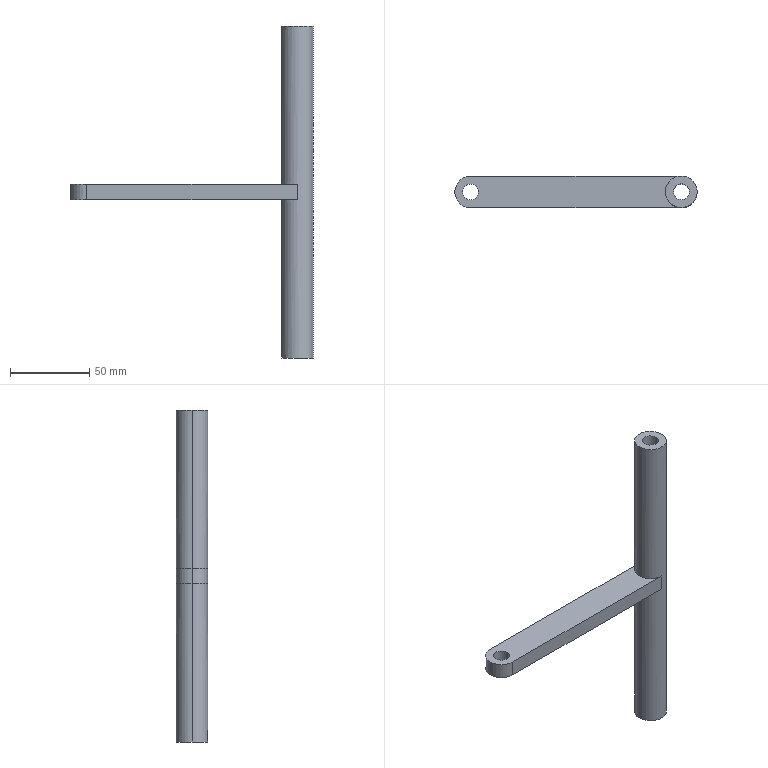Part | SolidWorks | features ICE 3, Extrusion 1 | 1 solid | 14 faces | box 153.27 x 20 x 210 mm | volume 75349 mm3 | cylinder 8 | plane 6 | commonest cylinder face diameters 10 x4 20 x4
STEP:
#1=CARTESIAN_POINT('',(71.635,0.,110.));
#2=VERTEX_POINT('',#1);
#3=CARTESIAN_POINT('',(61.635,0.,110.));
#4=VERTEX_POINT('',#3);
#5=CARTESIAN_POINT('',(66.635,0.,110.));
#6=DIRECTION('',(0.,0.,-1.));
#7=DIRECTION('',(-1.,0.,0.));
#8=AXIS2_PLACEMENT_3D('',#5,#6,#7);
#9=CIRCLE('',#8,5.);
#10=EDGE_CURVE('',#2,#4,#9,.T.);
#11=ORIENTED_EDGE('',*,*,#10,.F.);
#12=CARTESIAN_POINT('',(71.635,0.,-100.));
#13=VERTEX_POINT('',#12);
#14=CARTESIAN_POINT('',(71.635,0.,110.));
#15=DIRECTION('',(0.,0.,-1.));
#16=VECTOR('',#15,1000.);
#17=LINE('',#14,#16);
#18=EDGE_CURVE('',#2,#13,#17,.T.);
#19=ORIENTED_EDGE('',*,*,#18,.T.);
#20=CARTESIAN_POINT('',(61.635,0.,-100.));
#21=VERTEX_POINT('',#20);
#22=CARTESIAN_POINT('',(66.635,0.,-100.));
#23=DIRECTION('',(0.,0.,-1.));
#24=DIRECTION('',(-1.,0.,0.));
#25=AXIS2_PLACEMENT_3D('',#22,#23,#24);
#26=CIRCLE('',#25,5.);
#27=EDGE_CURVE('',#13,#21,#26,.T.);
#28=ORIENTED_EDGE('',*,*,#27,.T.);
#29=CARTESIAN_POINT('',(61.635,0.,110.));
#30=DIRECTION('',(0.,0.,-1.));
#31=VECTOR('',#30,1000.);
#32=LINE('',#29,#31);
#33=EDGE_CURVE('',#4,#21,#32,.T.);
#34=ORIENTED_EDGE('',*,*,#33,.F.);
#35=EDGE_LOOP('',(#11,#19,#28,#34));
#36=FACE_OUTER_BOUND('',#35,.T.);
#37=CARTESIAN_POINT('',(66.635,0.,110.));
#38=DIRECTION('',(0.,0.,-1.));
#39=DIRECTION('',(-1.,0.,0.));
#40=AXIS2_PLACEMENT_3D('',#37,#38,#39);
#41=CYLINDRICAL_SURFACE('',#40,5.);
#42=ADVANCED_FACE('',(#36),#41,.F.);
#43=CARTESIAN_POINT('',(76.635,0.,110.));
#44=VERTEX_POINT('',#43);
#45=CARTESIAN_POINT('',(56.635,0.,110.));
#46=VERTEX_POINT('',#45);
#47=CARTESIAN_POINT('',(66.635,0.,110.));
#48=DIRECTION('',(0.,0.,1.));
#49=DIRECTION('',(1.,0.,0.));
#50=AXIS2_PLACEMENT_3D('',#47,#48,#49);
#51=CIRCLE('',#50,10.);
#52=EDGE_CURVE('',#44,#46,#51,.T.);
#53=ORIENTED_EDGE('',*,*,#52,.F.);
#54=CARTESIAN_POINT('',(76.635,0.,-100.));
#55=VERTEX_POINT('',#54);
#56=CARTESIAN_POINT('',(76.635,0.,10.));
#57=DIRECTION('',(0.,0.,-1.));
#58=VECTOR('',#57,1000.);
#59=LINE('',#56,#58);
#60=EDGE_CURVE('',#44,#55,#59,.T.);
#61=ORIENTED_EDGE('',*,*,#60,.T.);
#62=CARTESIAN_POINT('',(56.635,0.,-100.));
#63=VERTEX_POINT('',#62);
#64=CARTESIAN_POINT('',(66.635,0.,-100.));
#65=DIRECTION('',(0.,0.,-1.));
#66=DIRECTION('',(-1.,0.,0.));
#67=AXIS2_PLACEMENT_3D('',#64,#65,#66);
#68=CIRCLE('',#67,10.);
#69=EDGE_CURVE('',#63,#55,#68,.T.);
#70=ORIENTED_EDGE('',*,*,#69,.F.);
#71=CARTESIAN_POINT('',(56.635,0.,0.));
#72=VERTEX_POINT('',#71);
#73=CARTESIAN_POINT('',(56.635,0.,10.));
#74=DIRECTION('',(0.,0.,-1.));
#75=VECTOR('',#74,1000.);
#76=LINE('',#73,#75);
#77=EDGE_CURVE('',#72,#63,#76,.T.);
#78=ORIENTED_EDGE('',*,*,#77,.F.);
#79=CARTESIAN_POINT('',(66.635,10.,0.));
#80=VERTEX_POINT('',#79);
#81=CARTESIAN_POINT('',(66.635,0.,0.));
#82=DIRECTION('',(0.,0.,-1.));
#83=DIRECTION('',(-1.,0.,0.));
#84=AXIS2_PLACEMENT_3D('',#81,#82,#83);
#85=CIRCLE('',#84,10.);
#86=EDGE_CURVE('',#72,#80,#85,.T.);
#87=ORIENTED_EDGE('',*,*,#86,.T.);
#88=CARTESIAN_POINT('',(66.635,10.,10.));
#89=VERTEX_POINT('',#88);
#90=CARTESIAN_POINT('',(66.635,10.,10.));
#91=DIRECTION('',(0.,0.,-1.));
#92=VECTOR('',#91,1000.);
#93=LINE('',#90,#92);
#94=EDGE_CURVE('',#89,#80,#93,.T.);
#95=ORIENTED_EDGE('',*,*,#94,.F.);
#96=CARTESIAN_POINT('',(56.635,0.,10.));
#97=VERTEX_POINT('',#96);
#98=CARTESIAN_POINT('',(66.635,0.,10.));
#99=DIRECTION('',(0.,0.,1.));
#100=DIRECTION('',(1.,0.,0.));
#101=AXIS2_PLACEMENT_3D('',#98,#99,#100);
#102=CIRCLE('',#101,10.);
#103=EDGE_CURVE('',#89,#97,#102,.T.);
#104=ORIENTED_EDGE('',*,*,#103,.T.);
#105=CARTESIAN_POINT('',(56.635,0.,10.));
#106=DIRECTION('',(0.,0.,-1.));
#107=VECTOR('',#106,1000.);
#108=LINE('',#105,#107);
#109=EDGE_CURVE('',#46,#97,#108,.T.);
#110=ORIENTED_EDGE('',*,*,#109,.F.);
#111=EDGE_LOOP('',(#53,#61,#70,#78,#87,#95,#104,#110));
#112=FACE_OUTER_BOUND('',#111,.T.);
#113=CARTESIAN_POINT('',(66.635,0.,10.));
#114=DIRECTION('',(0.,0.,-1.));
#115=DIRECTION('',(-1.,0.,0.));
#116=AXIS2_PLACEMENT_3D('',#113,#114,#115);
#117=CYLINDRICAL_SURFACE('',#116,10.);
#118=ADVANCED_FACE('',(#112),#117,.T.);
#119=CARTESIAN_POINT('',(-76.635,0.,10.));
#120=VERTEX_POINT('',#119);
#121=CARTESIAN_POINT('',(-66.635,-10.,10.));
#122=VERTEX_POINT('',#121);
#123=CARTESIAN_POINT('',(-66.635,0.,10.));
#124=DIRECTION('',(0.,0.,1.));
#125=DIRECTION('',(1.,0.,0.));
#126=AXIS2_PLACEMENT_3D('',#123,#124,#125);
#127=CIRCLE('',#126,10.);
#128=EDGE_CURVE('',#120,#122,#127,.T.);
#129=ORIENTED_EDGE('',*,*,#128,.F.);
#130=CARTESIAN_POINT('',(-76.635,0.,0.));
#131=VERTEX_POINT('',#130);
#132=CARTESIAN_POINT('',(-76.635,0.,10.));
#133=DIRECTION('',(0.,0.,-1.));
#134=VECTOR('',#133,1000.);
#135=LINE('',#132,#134);
#136=EDGE_CURVE('',#120,#131,#135,.T.);
#137=ORIENTED_EDGE('',*,*,#136,.T.);
#138=CARTESIAN_POINT('',(-66.635,-10.,0.));
#139=VERTEX_POINT('',#138);
#140=CARTESIAN_POINT('',(-66.635,0.,0.));
#141=DIRECTION('',(0.,0.,1.));
#142=DIRECTION('',(1.,0.,0.));
#143=AXIS2_PLACEMENT_3D('',#140,#141,#142);
#144=CIRCLE('',#143,10.);
#145=EDGE_CURVE('',#131,#139,#144,.T.);
#146=ORIENTED_EDGE('',*,*,#145,.T.);
#147=CARTESIAN_POINT('',(-66.635,-10.,10.));
#148=DIRECTION('',(0.,0.,-1.));
#149=VECTOR('',#148,1000.);
#150=LINE('',#147,#149);
#151=EDGE_CURVE('',#122,#139,#150,.T.);
#152=ORIENTED_EDGE('',*,*,#151,.F.);
#153=EDGE_LOOP('',(#129,#137,#146,#152));
#154=FACE_OUTER_BOUND('',#153,.T.);
#155=CARTESIAN_POINT('',(-66.635,0.,10.));
#156=DIRECTION('',(0.,0.,-1.));
#157=DIRECTION('',(-1.,0.,0.));
#158=AXIS2_PLACEMENT_3D('',#155,#156,#157);
#159=CYLINDRICAL_SURFACE('',#158,10.);
#160=ADVANCED_FACE('',(#154),#159,.T.);
#161=CARTESIAN_POINT('',(-71.635,0.,10.));
#162=VERTEX_POINT('',#161);
#163=CARTESIAN_POINT('',(-61.635,0.,10.));
#164=VERTEX_POINT('',#163);
#165=CARTESIAN_POINT('',(-66.635,0.,10.));
#166=DIRECTION('',(0.,0.,1.));
#167=DIRECTION('',(1.,0.,0.));
#168=AXIS2_PLACEMENT_3D('',#165,#166,#167);
#169=CIRCLE('',#168,5.);
#170=EDGE_CURVE('',#162,#164,#169,.T.);
#171=ORIENTED_EDGE('',*,*,#170,.T.);
#172=CARTESIAN_POINT('',(-61.635,0.,0.));
#173=VERTEX_POINT('',#172);
#174=CARTESIAN_POINT('',(-61.635,0.,10.));
#175=DIRECTION('',(0.,0.,-1.));
#176=VECTOR('',#175,1000.);
#177=LINE('',#174,#176);
#178=EDGE_CURVE('',#164,#173,#177,.T.);
#179=ORIENTED_EDGE('',*,*,#178,.T.);
#180=CARTESIAN_POINT('',(-71.635,0.,0.));
#181=VERTEX_POINT('',#180);
#182=CARTESIAN_POINT('',(-66.635,0.,0.));
#183=DIRECTION('',(0.,0.,1.));
#184=DIRECTION('',(1.,0.,0.));
#185=AXIS2_PLACEMENT_3D('',#182,#183,#184);
#186=CIRCLE('',#185,5.);
#187=EDGE_CURVE('',#181,#173,#186,.T.);
#188=ORIENTED_EDGE('',*,*,#187,.F.);
#189=CARTESIAN_POINT('',(-71.635,0.,10.));
#190=DIRECTION('',(0.,0.,-1.));
#191=VECTOR('',#190,1000.);
#192=LINE('',#189,#191);
#193=EDGE_CURVE('',#162,#181,#192,.T.);
#194=ORIENTED_EDGE('',*,*,#193,.F.);
#195=EDGE_LOOP('',(#171,#179,#188,#194));
#196=FACE_OUTER_BOUND('',#195,.T.);
#197=CARTESIAN_POINT('',(-66.635,0.,10.));
#198=DIRECTION('',(0.,0.,-1.));
#199=DIRECTION('',(-1.,0.,0.));
#200=AXIS2_PLACEMENT_3D('',#197,#198,#199);
#201=CYLINDRICAL_SURFACE('',#200,5.);
#202=ADVANCED_FACE('',(#196),#201,.F.);
#203=CARTESIAN_POINT('',(66.635,0.,-100.));
#204=DIRECTION('',(0.,0.,-1.));
#205=DIRECTION('',(-1.,0.,0.));
#206=AXIS2_PLACEMENT_3D('',#203,#204,#205);
#207=CIRCLE('',#206,5.);
#208=EDGE_CURVE('',#21,#13,#207,.T.);
#209=ORIENTED_EDGE('',*,*,#208,.F.);
#210=ORIENTED_EDGE('',*,*,#27,.F.);
#211=EDGE_LOOP('',(#209,#210));
#212=FACE_BOUND('',#211,.T.);
#213=ORIENTED_EDGE('',*,*,#69,.T.);
#214=CARTESIAN_POINT('',(66.635,0.,-100.));
#215=DIRECTION('',(0.,0.,-1.));
#216=DIRECTION('',(-1.,0.,0.));
#217=AXIS2_PLACEMENT_3D('',#214,#215,#216);
#218=CIRCLE('',#217,10.);
#219=EDGE_CURVE('',#55,#63,#218,.T.);
#220=ORIENTED_EDGE('',*,*,#219,.T.);
#221=EDGE_LOOP('',(#213,#220));
#222=FACE_OUTER_BOUND('',#221,.T.);
#223=CARTESIAN_POINT('',(66.635,0.,-100.));
#224=DIRECTION('',(0.,0.,-1.));
#225=DIRECTION('',(-1.,0.,0.));
#226=AXIS2_PLACEMENT_3D('',#223,#224,#225);
#227=PLANE('',#226);
#228=ADVANCED_FACE('',(#212,#222),#227,.T.);
#229=CARTESIAN_POINT('',(66.635,0.,110.));
#230=DIRECTION('',(0.,0.,-1.));
#231=DIRECTION('',(-1.,0.,0.));
#232=AXIS2_PLACEMENT_3D('',#229,#230,#231);
#233=CIRCLE('',#232,5.);
#234=EDGE_CURVE('',#4,#2,#233,.T.);
#235=ORIENTED_EDGE('',*,*,#234,.T.);
#236=ORIENTED_EDGE('',*,*,#10,.T.);
#237=EDGE_LOOP('',(#235,#236));
#238=FACE_BOUND('',#237,.T.);
#239=CARTESIAN_POINT('',(66.635,0.,110.));
#240=DIRECTION('',(0.,0.,1.));
#241=DIRECTION('',(1.,0.,0.));
#242=AXIS2_PLACEMENT_3D('',#239,#240,#241);
#243=CIRCLE('',#242,10.);
#244=EDGE_CURVE('',#46,#44,#243,.T.);
#245=ORIENTED_EDGE('',*,*,#244,.T.);
#246=ORIENTED_EDGE('',*,*,#52,.T.);
#247=EDGE_LOOP('',(#245,#246));
#248=FACE_OUTER_BOUND('',#247,.T.);
#249=CARTESIAN_POINT('',(66.635,0.,110.));
#250=DIRECTION('',(0.,0.,1.));
#251=DIRECTION('',(1.,0.,0.));
#252=AXIS2_PLACEMENT_3D('',#249,#250,#251);
#253=PLANE('',#252);
#254=ADVANCED_FACE('',(#238,#248),#253,.T.);
#255=ORIENTED_EDGE('',*,*,#103,.F.);
#256=CARTESIAN_POINT('',(-66.635,10.,10.));
#257=VERTEX_POINT('',#256);
#258=CARTESIAN_POINT('',(-66.635,10.,10.));
#259=DIRECTION('',(-1.,0.,0.));
#260=VECTOR('',#259,1000.);
#261=LINE('',#258,#260);
#262=EDGE_CURVE('',#89,#257,#261,.T.);
#263=ORIENTED_EDGE('',*,*,#262,.T.);
#264=CARTESIAN_POINT('',(-66.635,0.,10.));
#265=DIRECTION('',(0.,0.,1.));
#266=DIRECTION('',(1.,0.,0.));
#267=AXIS2_PLACEMENT_3D('',#264,#265,#266);
#268=CIRCLE('',#267,10.);
#269=EDGE_CURVE('',#257,#120,#268,.T.);
#270=ORIENTED_EDGE('',*,*,#269,.T.);
#271=ORIENTED_EDGE('',*,*,#128,.T.);
#272=CARTESIAN_POINT('',(66.635,-10.,10.));
#273=VERTEX_POINT('',#272);
#274=CARTESIAN_POINT('',(-66.635,-10.,10.));
#275=DIRECTION('',(1.,0.,0.));
#276=VECTOR('',#275,1000.);
#277=LINE('',#274,#276);
#278=EDGE_CURVE('',#122,#273,#277,.T.);
#279=ORIENTED_EDGE('',*,*,#278,.T.);
#280=CARTESIAN_POINT('',(66.635,0.,10.));
#281=DIRECTION('',(0.,0.,1.));
#282=DIRECTION('',(1.,0.,0.));
#283=AXIS2_PLACEMENT_3D('',#280,#281,#282);
#284=CIRCLE('',#283,10.);
#285=EDGE_CURVE('',#97,#273,#284,.T.);
#286=ORIENTED_EDGE('',*,*,#285,.F.);
#287=EDGE_LOOP('',(#255,#263,#270,#271,#279,#286));
#288=FACE_OUTER_BOUND('',#287,.T.);
#289=ORIENTED_EDGE('',*,*,#170,.F.);
#290=CARTESIAN_POINT('',(-66.635,0.,10.));
#291=DIRECTION('',(0.,0.,1.));
#292=DIRECTION('',(1.,0.,0.));
#293=AXIS2_PLACEMENT_3D('',#290,#291,#292);
#294=CIRCLE('',#293,5.);
#295=EDGE_CURVE('',#164,#162,#294,.T.);
#296=ORIENTED_EDGE('',*,*,#295,.F.);
#297=EDGE_LOOP('',(#289,#296));
#298=FACE_BOUND('',#297,.T.);
#299=CARTESIAN_POINT('',(-66.635,0.,10.));
#300=DIRECTION('',(0.,0.,1.));
#301=DIRECTION('',(1.,0.,0.));
#302=AXIS2_PLACEMENT_3D('',#299,#300,#301);
#303=PLANE('',#302);
#304=ADVANCED_FACE('',(#288,#298),#303,.T.);
#305=ORIENTED_EDGE('',*,*,#178,.F.);
#306=ORIENTED_EDGE('',*,*,#295,.T.);
#307=ORIENTED_EDGE('',*,*,#193,.T.);
#308=CARTESIAN_POINT('',(-66.635,0.,0.));
#309=DIRECTION('',(0.,0.,1.));
#310=DIRECTION('',(1.,0.,0.));
#311=AXIS2_PLACEMENT_3D('',#308,#309,#310);
#312=CIRCLE('',#311,5.);
#313=EDGE_CURVE('',#173,#181,#312,.T.);
#314=ORIENTED_EDGE('',*,*,#313,.F.);
#315=EDGE_LOOP('',(#305,#306,#307,#314));
#316=FACE_OUTER_BOUND('',#315,.T.);
#317=CARTESIAN_POINT('',(-66.635,0.,10.));
#318=DIRECTION('',(0.,0.,-1.));
#319=DIRECTION('',(-1.,0.,0.));
#320=AXIS2_PLACEMENT_3D('',#317,#318,#319);
#321=CYLINDRICAL_SURFACE('',#320,5.);
#322=ADVANCED_FACE('',(#316),#321,.F.);
#323=CARTESIAN_POINT('',(-66.635,10.,0.));
#324=VERTEX_POINT('',#323);
#325=CARTESIAN_POINT('',(-66.635,10.,0.));
#326=DIRECTION('',(-1.,0.,0.));
#327=VECTOR('',#326,1000.);
#328=LINE('',#325,#327);
#329=EDGE_CURVE('',#80,#324,#328,.T.);
#330=ORIENTED_EDGE('',*,*,#329,.T.);
#331=CARTESIAN_POINT('',(-66.635,10.,10.));
#332=DIRECTION('',(0.,0.,-1.));
#333=VECTOR('',#332,1000.);
#334=LINE('',#331,#333);
#335=EDGE_CURVE('',#257,#324,#334,.T.);
#336=ORIENTED_EDGE('',*,*,#335,.F.);
#337=ORIENTED_EDGE('',*,*,#262,.F.);
#338=ORIENTED_EDGE('',*,*,#94,.T.);
#339=EDGE_LOOP('',(#330,#336,#337,#338));
#340=FACE_OUTER_BOUND('',#339,.T.);
#341=CARTESIAN_POINT('',(-66.635,10.,10.));
#342=DIRECTION('',(0.,-1.,0.));
#343=DIRECTION('',(0.,0.,-1.));
#344=AXIS2_PLACEMENT_3D('',#341,#342,#343);
#345=PLANE('',#344);
#346=ADVANCED_FACE('',(#340),#345,.F.);
#347=ORIENTED_EDGE('',*,*,#136,.F.);
#348=ORIENTED_EDGE('',*,*,#269,.F.);
#349=ORIENTED_EDGE('',*,*,#335,.T.);
#350=CARTESIAN_POINT('',(-66.635,0.,0.));
#351=DIRECTION('',(0.,0.,1.));
#352=DIRECTION('',(1.,0.,0.));
#353=AXIS2_PLACEMENT_3D('',#350,#351,#352);
#354=CIRCLE('',#353,10.);
#355=EDGE_CURVE('',#324,#131,#354,.T.);
#356=ORIENTED_EDGE('',*,*,#355,.T.);
#357=EDGE_LOOP('',(#347,#348,#349,#356));
#358=FACE_OUTER_BOUND('',#357,.T.);
#359=CARTESIAN_POINT('',(-66.635,0.,10.));
#360=DIRECTION('',(0.,0.,-1.));
#361=DIRECTION('',(-1.,0.,0.));
#362=AXIS2_PLACEMENT_3D('',#359,#360,#361);
#363=CYLINDRICAL_SURFACE('',#362,10.);
#364=ADVANCED_FACE('',(#358),#363,.T.);
#365=ORIENTED_EDGE('',*,*,#60,.F.);
#366=ORIENTED_EDGE('',*,*,#244,.F.);
#367=ORIENTED_EDGE('',*,*,#109,.T.);
#368=ORIENTED_EDGE('',*,*,#285,.T.);
#369=CARTESIAN_POINT('',(66.635,-10.,0.));
#370=VERTEX_POINT('',#369);
#371=CARTESIAN_POINT('',(66.635,-10.,10.));
#372=DIRECTION('',(0.,0.,-1.));
#373=VECTOR('',#372,1000.);
#374=LINE('',#371,#373);
#375=EDGE_CURVE('',#273,#370,#374,.T.);
#376=ORIENTED_EDGE('',*,*,#375,.T.);
#377=CARTESIAN_POINT('',(66.635,0.,0.));
#378=DIRECTION('',(0.,0.,-1.));
#379=DIRECTION('',(-1.,0.,0.));
#380=AXIS2_PLACEMENT_3D('',#377,#378,#379);
#381=CIRCLE('',#380,10.);
#382=EDGE_CURVE('',#370,#72,#381,.T.);
#383=ORIENTED_EDGE('',*,*,#382,.T.);
#384=ORIENTED_EDGE('',*,*,#77,.T.);
#385=ORIENTED_EDGE('',*,*,#219,.F.);
#386=EDGE_LOOP('',(#365,#366,#367,#368,#376,#383,#384,#385));
#387=FACE_OUTER_BOUND('',#386,.T.);
#388=CARTESIAN_POINT('',(66.635,0.,10.));
#389=DIRECTION('',(0.,0.,-1.));
#390=DIRECTION('',(-1.,0.,0.));
#391=AXIS2_PLACEMENT_3D('',#388,#389,#390);
#392=CYLINDRICAL_SURFACE('',#391,10.);
#393=ADVANCED_FACE('',(#387),#392,.T.);
#394=CARTESIAN_POINT('',(-66.635,-10.,0.));
#395=DIRECTION('',(1.,0.,0.));
#396=VECTOR('',#395,1000.);
#397=LINE('',#394,#396);
#398=EDGE_CURVE('',#139,#370,#397,.T.);
#399=ORIENTED_EDGE('',*,*,#398,.T.);
#400=ORIENTED_EDGE('',*,*,#375,.F.);
#401=ORIENTED_EDGE('',*,*,#278,.F.);
#402=ORIENTED_EDGE('',*,*,#151,.T.);
#403=EDGE_LOOP('',(#399,#400,#401,#402));
#404=FACE_OUTER_BOUND('',#403,.T.);
#405=CARTESIAN_POINT('',(-66.635,-10.,10.));
#406=DIRECTION('',(0.,1.,0.));
#407=DIRECTION('',(0.,0.,1.));
#408=AXIS2_PLACEMENT_3D('',#405,#406,#407);
#409=PLANE('',#408);
#410=ADVANCED_FACE('',(#404),#409,.F.);
#411=ORIENTED_EDGE('',*,*,#382,.F.);
#412=ORIENTED_EDGE('',*,*,#398,.F.);
#413=ORIENTED_EDGE('',*,*,#145,.F.);
#414=ORIENTED_EDGE('',*,*,#355,.F.);
#415=ORIENTED_EDGE('',*,*,#329,.F.);
#416=ORIENTED_EDGE('',*,*,#86,.F.);
#417=EDGE_LOOP('',(#411,#412,#413,#414,#415,#416));
#418=FACE_OUTER_BOUND('',#417,.T.);
#419=ORIENTED_EDGE('',*,*,#187,.T.);
#420=ORIENTED_EDGE('',*,*,#313,.T.);
#421=EDGE_LOOP('',(#419,#420));
#422=FACE_BOUND('',#421,.T.);
#423=CARTESIAN_POINT('',(-66.635,0.,0.));
#424=DIRECTION('',(0.,0.,1.));
#425=DIRECTION('',(1.,0.,0.));
#426=AXIS2_PLACEMENT_3D('',#423,#424,#425);
#427=PLANE('',#426);
#428=ADVANCED_FACE('',(#418,#422),#427,.F.);
#429=ORIENTED_EDGE('',*,*,#18,.F.);
#430=ORIENTED_EDGE('',*,*,#234,.F.);
#431=ORIENTED_EDGE('',*,*,#33,.T.);
#432=ORIENTED_EDGE('',*,*,#208,.T.);
#433=EDGE_LOOP('',(#429,#430,#431,#432));
#434=FACE_OUTER_BOUND('',#433,.T.);
#435=CARTESIAN_POINT('',(66.635,0.,110.));
#436=DIRECTION('',(0.,0.,-1.));
#437=DIRECTION('',(-1.,0.,0.));
#438=AXIS2_PLACEMENT_3D('',#435,#436,#437);
#439=CYLINDRICAL_SURFACE('',#438,5.);
#440=ADVANCED_FACE('',(#434),#439,.F.);
#441=CLOSED_SHELL('',(#42,#118,#160,#202,#228,#254,#304,#322,#346,#364,#393,#410,#428,#440));
#442=MANIFOLD_SOLID_BREP('',#441);
#443=CARTESIAN_POINT('',(0.,0.,0.));
#444=DIRECTION('',(0.,0.,1.));
#445=DIRECTION('',(1.,0.,0.));
#446=AXIS2_PLACEMENT_3D('',#443,#444,#445);
#447=(LENGTH_UNIT()NAMED_UNIT(*)SI_UNIT(.MILLI.,.METRE.));
#448=UNCERTAINTY_MEASURE_WITH_UNIT(LENGTH_MEASURE(0.00001),#447,'','');
#449=(NAMED_UNIT(*)PLANE_ANGLE_UNIT()SI_UNIT($,.RADIAN.));
#450=(NAMED_UNIT(*)SI_UNIT($,.STERADIAN.)SOLID_ANGLE_UNIT());
#451=(GEOMETRIC_REPRESENTATION_CONTEXT(3)GLOBAL_UNCERTAINTY_ASSIGNED_CONTEXT((#448))GLOBAL_UNIT_ASSIGNED_CONTEXT((#447,#449,#450))REPRESENTATION_CONTEXT('',''));
#452=ADVANCED_BREP_SHAPE_REPRESENTATION('',(#442,#446),#451);